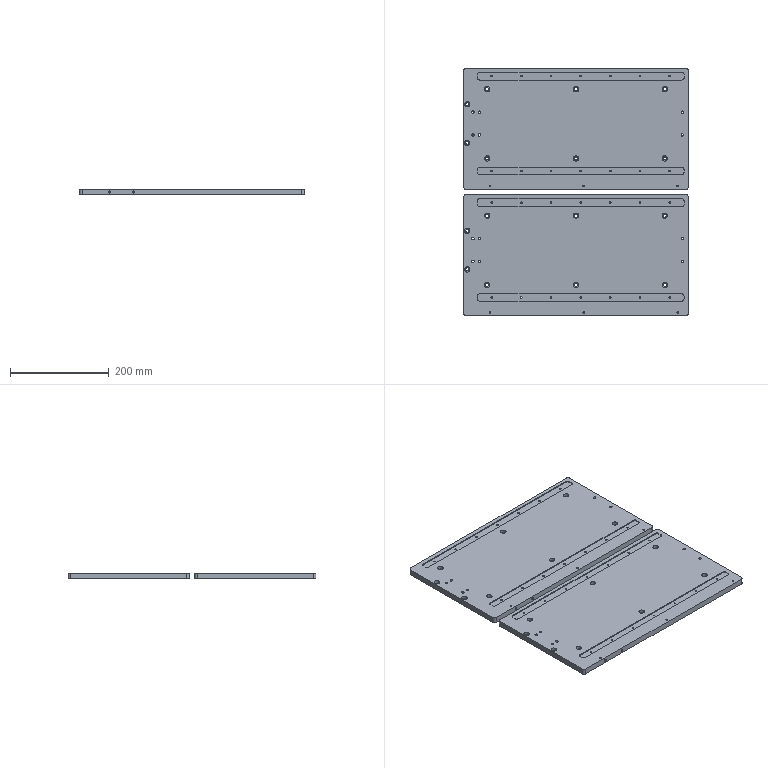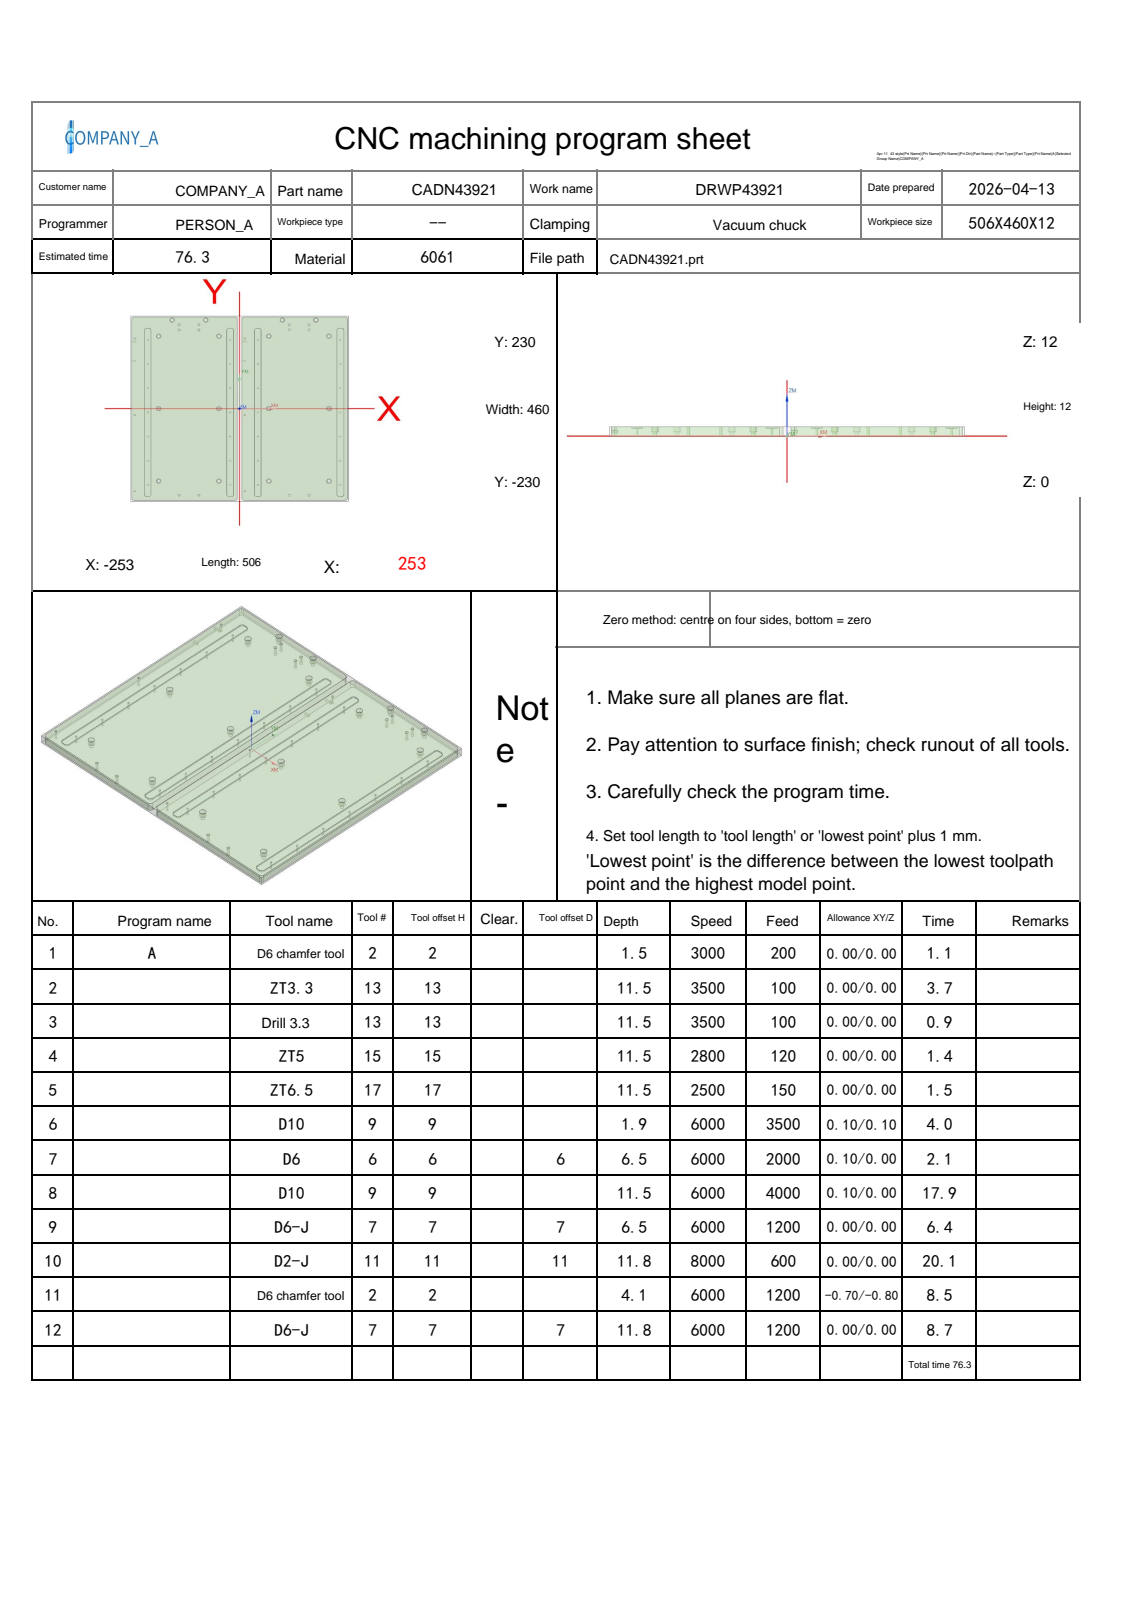NC program | NX | posted by the shop | part box 455 x 501 x 12 mm
Lines 1 to 1767 of 11580, first 1628 of 1765 lines:
%
O0001
(Machine time: 77.93 MIN)
(===Total Tool:8===)
(T2=D6 chamfer tool   D=6.   R=0.   D-  H02 Z=7.85  )
(T13=ZT3.3  D=3.3  DR_a=118 D-  H13 Z=0.5   )
(T15=ZT5    D=5.   DR_a=118 D-  H15 Z=0.5   )
(T17=ZT6.5  D=6.5  DR_a=118 D-  H17 Z=0.5   )
(T9=D10     D=10.  R=0.   D-  H09 Z=0.5   )
(T6=D6      D=6.   R=0.   D6  H06 Z=5.5   )
(T7=D6-J    D=6.   R=0.   D7  H07 Z=0.2   )
(T11=D2-J   D=2.   R=0.   D11 H11 Z=0.2   )
G80 G90 G17 G49 G40
G91 G28 Z0
M01
N1 T02 M06
(D6 chamfer tool  D=6. R=0. H=02 ce=0.00 di=0.00)
G00 G90 G54 X42.5 Y-129.5 M03 S3000
G43 H02 Z32.
M08
G98 G81 X42.5 Y-129.5 Z10.5 R13. F200.
Y-69.5
X12. Y-15.678
X42.5 Y-9.5
X68. Y0.0
X42.5 Y50.5
Y110.5
X-21.5
Y50.5
X-48. Y0.0
X-21.5 Y-9.5
Y-69.5
Y-129.5
X-48. Y-180.
X-21.5 Y-189.5
X12. Y-205.678
X42.5 Y-189.5
X68. Y-180.
X115.5 Y-215.
X161.5
X208. Y-180.
X234.5 Y-189.5
Y-129.5
Y-69.5
Y-9.5
X208. Y0.0
X234.5 Y50.5
Y110.5
Y170.5
X208. Y180.
X177.5 Y220.
X161.5 Y208.5
Y195.5
X115.5
Y208.5
X99.5 Y220.
X68. Y180.
X42.5 Y170.5
X12. Y174.322
X-21.5 Y170.5
X-48. Y180.
X-78.5 Y220.
X-94.5 Y208.5
Y195.5
X-140.5
Y208.5
X-156.5 Y220.
X-188. Y180.
X-213.5 Y170.5
X-244. Y174.322
X-213.5 Y110.5
Y50.5
X-188. Y0.0
X-213.5 Y-9.5
X-244. Y-15.678
X-213.5 Y-69.5
Y-129.5
X-244. Y-205.678
X-213.5 Y-189.5
X-188. Y-180.
X-140.5 Y-215.
X-94.5
G80
G00 Z32.
G91 G28 Z0.0
M05
M09
G91 G28 Z0.0
M01
N2 T13 M06
(ZT3.3 D=3.3 DR_a=118 H=13)
G00 G90 G54 X-213.5 Y-189.5 M03 S3500
G43 H13 Z32.
M08
G98 G83 X-213.5 Y-189.5 Z.5 R13. F100. Q1.5
Y-129.5
Y-69.5
Y-9.5
Y50.5
Y110.5
Y170.5
X-21.5 Y110.5
Y170.5
X42.5
Y110.5
Y50.5
X-21.5
Y-9.5
X42.5
Y-69.5
X-21.5
Y-129.5
Y-189.5
X42.5
Y-129.5
X234.5 Y-189.5
Y-129.5
Y-69.5
Y-9.5
Y50.5
Y110.5
Y170.5
G80
G00 Z32.
G91 G28 Z0.0
M05
M09
G91 G28 Z0.0
M01
N3 T13 M06
(Drill 3.3 D=3.3 DR_a=118 H=13)
G00 G90 G54 X-244. Y-205.678 M03 S3500
G43 H13 Z32.
M08
G98 G83 X-244. Y-205.678 Z.5 R13. F100. Q1.5
Y-15.678
Y174.322
X12.
Y-15.678
Y-205.678
G80
G00 Z32.
G91 G28 Z0.0
M05
M09
G91 G28 Z0.0
M01
N4 T15 M06
(ZT5 D=5. DR_a=118 H=15)
G00 G90 G54 X161.5 Y195.5 M03 S2800
G43 H15 Z32.
M08
G98 G83 X161.5 Y195.5 Z.5 R13. F120. Q1.5
Y208.5
X115.5
Y195.5
X-94.5
Y208.5
X-140.5
Y195.5
Y-215.
X-94.5
X115.5
X161.5
G80
G00 Z32.
G91 G28 Z0.0
M05
M09
G91 G28 Z0.0
M01
N5 T17 M06
(ZT6.5 D=6.5 DR_a=118 H=17)
G00 G90 G54 X-188. Y180. M03 S2500
G43 H17 Z32.
M08
G98 G83 X-188. Y180. Z.5 R13. F150. Q3.
X-156.5 Y220.
X-78.5
X-48. Y180.
X68.
X99.5 Y220.
X177.5
X208. Y180.
Y0.0
X68.
X-48.
X-188.
Y-180.
X-48.
X68.
X208.
G80
G00 Z32.
G91 G28 Z0.0
M05
M09
G91 G28 Z0.0
M01
N6 T09 M06
(D10  D=10. R=0. H=09 ce=0.10 di=0.10)
G00 G90 G54 X237.1 Y-37.42 M03 S6000
G43 H09 Z32.
M08
Z12.5
M03 S6000
G01 Y-9.5 Z11.525 F2800.
X237.4
M03 S6000
Y194.5 F3500.
X237.395 Y194.555
X237.355 Y194.595
X237.3 Y194.6
X231.689 Y194.599
X231.638 Y194.591
X231.603 Y194.551
X231.6 Y194.5
Y-213.5
X231.605 Y-213.555
X231.645 Y-213.595
X231.7 Y-213.6
X237.3
X237.355 Y-213.595
X237.395 Y-213.555
X237.4 Y-213.5
Y-9.5
Z12.525
G00 Z13.
X237.1 Y-37.42
Z12.025
M03 S6000
G01 Y-9.5 Z11.05 F2800.
X237.4
M03 S6000
Y194.5 F3500.
X237.395 Y194.555
X237.355 Y194.595
X237.3 Y194.6
X231.689 Y194.599
X231.638 Y194.591
X231.603 Y194.551
X231.6 Y194.5
Y-213.5
X231.605 Y-213.555
X231.645 Y-213.595
X231.7 Y-213.6
X237.3
X237.355 Y-213.595
X237.395 Y-213.555
X237.4 Y-213.5
Y-9.5
Z12.05
G00 Z12.525
X237.1 Y-37.42
Z11.55
M03 S6000
G01 Y-9.5 Z10.575 F2800.
X237.4
M03 S6000
Y194.5 F3500.
X237.395 Y194.555
X237.355 Y194.595
X237.3 Y194.6
X231.689 Y194.599
X231.638 Y194.591
X231.603 Y194.551
X231.6 Y194.5
Y-213.5
X231.605 Y-213.555
X231.645 Y-213.595
X231.7 Y-213.6
X237.3
X237.355 Y-213.595
X237.395 Y-213.555
X237.4 Y-213.5
Y-9.5
Z11.575
G00 Z12.05
X237.1 Y-37.42
Z11.075
M03 S6000
G01 Y-9.5 Z10.1 F2800.
X237.4
M03 S6000
Y194.5 F3500.
X237.395 Y194.555
X237.355 Y194.595
X237.3 Y194.6
X231.689 Y194.599
X231.638 Y194.591
X231.603 Y194.551
X231.6 Y194.5
Y-213.5
X231.605 Y-213.555
X231.645 Y-213.595
X231.7 Y-213.6
X237.3
X237.355 Y-213.595
X237.395 Y-213.555
X237.4 Y-213.5
Y-9.5
Z11.1
G00 Z32.
X44.65 Y-37.42
Z12.5
M03 S6000
G01 Y-9.5 Z11.525 F2800.
X44.95
M03 S6000
Y194.45 F3500.
X40.05
Y-213.45
X44.95
Y-9.5
Z12.525
G00 Z13.
X44.65 Y-37.42
Z12.025
M03 S6000
G01 Y-9.5 Z11.05 F2800.
X44.95
M03 S6000
Y194.45 F3500.
X40.05
Y-213.45
X44.95
Y-9.5
Z12.05
G00 Z12.525
X44.65 Y-37.42
Z11.55
M03 S6000
G01 Y-9.5 Z10.575 F2800.
X44.95
M03 S6000
Y194.45 F3500.
X40.05
Y-213.45
X44.95
Y-9.5
Z11.575
G00 Z12.05
X44.65 Y-37.42
Z11.075
M03 S6000
G01 Y-9.5 Z10.1 F2800.
X44.95
M03 S6000
Y194.45 F3500.
X40.05
Y-213.45
X44.95
Y-9.5
Z11.1
G00 Z32.
X-18.9 Y-37.42
Z12.5
M03 S6000
G01 Y-9.5 Z11.525 F2800.
X-18.6
M03 S6000
Y194.5 F3500.
X-18.605 Y194.555
X-18.645 Y194.595
X-18.7 Y194.6
X-24.3
X-24.355 Y194.595
X-24.395 Y194.555
X-24.4 Y194.5
Y-213.5
X-24.403 Y-213.539
X-24.375 Y-213.567
X-24.357 Y-213.594
X-24.328 Y-213.606
X-24.296 Y-213.6
X-18.7
X-18.645 Y-213.595
X-18.605 Y-213.555
X-18.6 Y-213.5
Y-9.5
Z12.525
G00 Z13.
X-18.9 Y-37.42
Z12.025
M03 S6000
G01 Y-9.5 Z11.05 F2800.
X-18.6
M03 S6000
Y194.5 F3500.
X-18.605 Y194.555
X-18.645 Y194.595
X-18.7 Y194.6
X-24.3
X-24.355 Y194.595
X-24.395 Y194.555
X-24.4 Y194.5
Y-213.5
X-24.395 Y-213.555
X-24.355 Y-213.595
X-24.3 Y-213.6
X-18.7
X-18.645 Y-213.595
X-18.605 Y-213.555
X-18.6 Y-213.5
Y-9.5
Z12.05
G00 Z12.525
X-18.9 Y-37.42
Z11.55
M03 S6000
G01 Y-9.5 Z10.575 F2800.
X-18.6
M03 S6000
Y194.5 F3500.
X-18.605 Y194.555
X-18.645 Y194.595
X-18.7 Y194.6
X-24.3
X-24.355 Y194.595
X-24.395 Y194.555
X-24.4 Y194.5
Y-213.5
X-24.395 Y-213.555
X-24.355 Y-213.595
X-24.3 Y-213.6
X-18.7
X-18.645 Y-213.595
X-18.605 Y-213.555
X-18.6 Y-213.5
Y-9.5
Z11.575
G00 Z12.05
X-18.9 Y-37.42
Z11.075
M03 S6000
G01 Y-9.5 Z10.1 F2800.
X-18.6
M03 S6000
Y194.5 F3500.
X-18.605 Y194.555
X-18.645 Y194.595
X-18.7 Y194.6
X-24.3
X-24.355 Y194.595
X-24.395 Y194.555
X-24.4 Y194.5
Y-213.5
X-24.395 Y-213.555
X-24.355 Y-213.595
X-24.3 Y-213.6
X-18.7
X-18.645 Y-213.595
X-18.605 Y-213.555
X-18.6 Y-213.5
Y-9.5
Z11.1
G00 Z32.
X-215.65 Y18.42
Z12.5
M03 S6000
G01 Y-9.5 Z11.525 F2800.
X-215.95
M03 S6000
Y-213.45 F3500.
X-211.05
Y194.45
X-215.95
Y-9.5
Z12.525
G00 Z13.
X-215.65 Y18.42
Z12.025
M03 S6000
G01 Y-9.5 Z11.05 F2800.
X-215.95
M03 S6000
Y-213.45 F3500.
X-211.05
Y194.45
X-215.95
Y-9.5
Z12.05
G00 Z12.525
X-215.65 Y18.42
Z11.55
M03 S6000
G01 Y-9.5 Z10.575 F2800.
X-215.95
M03 S6000
Y-213.45 F3500.
X-211.05
Y194.45
X-215.95
Y-9.5
Z11.575
G00 Z12.05
X-215.65 Y18.42
Z11.075
M03 S6000
G01 Y-9.5 Z10.1 F2800.
X-215.95
M03 S6000
Y-213.45 F3500.
X-211.05
Y194.45
X-215.95
Y-9.5
Z11.1
G00 Z32.
G91 G28 Z0.0
M05
M09
G91 G28 Z0.0
M01
N7 T06 M06
(D6  D=6. R=0. H=06 ce=0.10 di=0.00)
G00 G90 G54 X-156.5 Y220. M03 S6000
G43 H06 Z32.
M08
Z12.3
G41 D06
G01 X-156.6 Y219.992 F2000.
G03 X-157.698 Y218.798 I.1 J-1.194
X-156.5 Y217.6 I1.198 J0.0
X-156.5 Y217.6 Z11.8 I0.0 J2.4
X-156.5 Y217.6 Z11.3 I0.0 J2.4
X-156.5 Y217.6 Z10.8 I0.0 J2.4
X-156.5 Y217.6 Z10.3 I0.0 J2.4
X-156.5 Y217.6 Z9.8 I0.0 J2.4
X-156.5 Y217.6 Z9.3 I0.0 J2.4
X-156.5 Y217.6 Z8.8 I0.0 J2.4
X-156.5 Y217.6 Z8.3 I0.0 J2.4
X-156.5 Y217.6 Z7.8 I0.0 J2.4
X-156.5 Y217.6 Z7.3 I0.0 J2.4
X-156.5 Y217.6 Z6.8 I0.0 J2.4
X-156.5 Y217.6 Z6.3 I0.0 J2.4
X-156.5 Y217.6 Z5.8 I0.0 J2.4
X-157.911 Y221.942 Z5.5 I0.0 J2.4
X-158.9 Y220. I1.411 J-1.942
X-156.5 Y217.6 I2.4 J0.0
X-154.1 Y220. I0.0 J2.4
X-156.5 Y222.4 I-2.4 J0.0
X-157.911 Y221.942 I0.0 J-2.4
X-158.404 Y220.973 I.704 J-.969
X-157.207 Y219.775 I1.198 J0.0
X-156.586 Y219.948 I0.0 J1.198
G01 G40 X-156.5 Y220.
G00 Z32.
X-188. Y180.
Z12.3
G41 D06
G01 X-188.1 Y179.992
G03 X-189.198 Y178.798 I.1 J-1.194
X-188. Y177.6 I1.198 J0.0
X-188. Y177.6 Z11.8 I0.0 J2.4
X-188. Y177.6 Z11.3 I0.0 J2.4
X-188. Y177.6 Z10.8 I0.0 J2.4
X-188. Y177.6 Z10.3 I0.0 J2.4
X-188. Y177.6 Z9.8 I0.0 J2.4
X-188. Y177.6 Z9.3 I0.0 J2.4
X-188. Y177.6 Z8.8 I0.0 J2.4
X-188. Y177.6 Z8.3 I0.0 J2.4
X-188. Y177.6 Z7.8 I0.0 J2.4
X-188. Y177.6 Z7.3 I0.0 J2.4
X-188. Y177.6 Z6.8 I0.0 J2.4
X-188. Y177.6 Z6.3 I0.0 J2.4
X-188. Y177.6 Z5.8 I0.0 J2.4
X-189.411 Y181.942 Z5.5 I0.0 J2.4
X-190.4 Y180. I1.411 J-1.942
X-188. Y177.6 I2.4 J0.0
X-185.6 Y180. I0.0 J2.4
X-188. Y182.4 I-2.4 J0.0
X-189.411 Y181.942 I0.0 J-2.4
X-189.904 Y180.973 I.704 J-.969
X-188.707 Y179.775 I1.198 J0.0
X-188.086 Y179.948 I0.0 J1.198
G01 G40 X-188. Y180.
G00 Z32.
X-78.5 Y220.
Z12.3
G41 D06
G01 X-78.6 Y219.992
G03 X-79.698 Y218.798 I.1 J-1.194
X-78.5 Y217.6 I1.198 J0.0
X-78.5 Y217.6 Z11.8 I0.0 J2.4
X-78.5 Y217.6 Z11.3 I0.0 J2.4
X-78.5 Y217.6 Z10.8 I0.0 J2.4
X-78.5 Y217.6 Z10.3 I0.0 J2.4
X-78.5 Y217.6 Z9.8 I0.0 J2.4
X-78.5 Y217.6 Z9.3 I0.0 J2.4
X-78.5 Y217.6 Z8.8 I0.0 J2.4
X-78.5 Y217.6 Z8.3 I0.0 J2.4
X-78.5 Y217.6 Z7.8 I0.0 J2.4
X-78.5 Y217.6 Z7.3 I0.0 J2.4
X-78.5 Y217.6 Z6.8 I0.0 J2.4
X-78.5 Y217.6 Z6.3 I0.0 J2.4
X-78.5 Y217.6 Z5.8 I0.0 J2.4
X-79.911 Y221.942 Z5.5 I0.0 J2.4
X-80.9 Y220. I1.411 J-1.942
X-78.5 Y217.6 I2.4 J0.0
X-76.1 Y220. I0.0 J2.4
X-78.5 Y222.4 I-2.4 J0.0
X-79.911 Y221.942 I0.0 J-2.4
X-80.404 Y220.973 I.704 J-.969
X-79.207 Y219.775 I1.198 J0.0
X-78.586 Y219.948 I0.0 J1.198
G01 G40 X-78.5 Y220.
G00 Z32.
X-48. Y180.
Z12.3
G41 D06
G01 X-48.1 Y179.992
G03 X-49.198 Y178.798 I.1 J-1.194
X-48. Y177.6 I1.198 J0.0
X-48. Y177.6 Z11.8 I0.0 J2.4
X-48. Y177.6 Z11.3 I0.0 J2.4
X-48. Y177.6 Z10.8 I0.0 J2.4
X-48. Y177.6 Z10.3 I0.0 J2.4
X-48. Y177.6 Z9.8 I0.0 J2.4
X-48. Y177.6 Z9.3 I0.0 J2.4
X-48. Y177.6 Z8.8 I0.0 J2.4
X-48. Y177.6 Z8.3 I0.0 J2.4
X-48. Y177.6 Z7.8 I0.0 J2.4
X-48. Y177.6 Z7.3 I0.0 J2.4
X-48. Y177.6 Z6.8 I0.0 J2.4
X-48. Y177.6 Z6.3 I0.0 J2.4
X-48. Y177.6 Z5.8 I0.0 J2.4
X-49.411 Y181.942 Z5.5 I0.0 J2.4
X-50.4 Y180. I1.411 J-1.942
X-48. Y177.6 I2.4 J0.0
X-45.6 Y180. I0.0 J2.4
X-48. Y182.4 I-2.4 J0.0
X-49.411 Y181.942 I0.0 J-2.4
X-49.904 Y180.973 I.704 J-.969
X-48.707 Y179.775 I1.198 J0.0
X-48.086 Y179.948 I0.0 J1.198
G01 G40 X-48. Y180.
G00 Z32.
X68.
Z12.3
G41 D06
G01 X67.9 Y179.992
G03 X66.802 Y178.798 I.1 J-1.194
X68. Y177.6 I1.198 J0.0
X68. Y177.6 Z11.8 I0.0 J2.4
X68. Y177.6 Z11.3 I0.0 J2.4
X68. Y177.6 Z10.8 I0.0 J2.4
X68. Y177.6 Z10.3 I0.0 J2.4
X68. Y177.6 Z9.8 I0.0 J2.4
X68. Y177.6 Z9.3 I0.0 J2.4
X68. Y177.6 Z8.8 I0.0 J2.4
X68. Y177.6 Z8.3 I0.0 J2.4
X68. Y177.6 Z7.8 I0.0 J2.4
X68. Y177.6 Z7.3 I0.0 J2.4
X68. Y177.6 Z6.8 I0.0 J2.4
X68. Y177.6 Z6.3 I0.0 J2.4
X68. Y177.6 Z5.8 I0.0 J2.4
X66.589 Y181.942 Z5.5 I0.0 J2.4
X65.6 Y180. I1.411 J-1.942
X68. Y177.6 I2.4 J0.0
X70.4 Y180. I0.0 J2.4
X68. Y182.4 I-2.4 J0.0
X66.589 Y181.942 I0.0 J-2.4
X66.096 Y180.973 I.704 J-.969
X67.293 Y179.775 I1.198 J0.0
X67.914 Y179.948 I0.0 J1.198
G01 G40 X68. Y180.
G00 Z32.
X99.5 Y220.
Z12.3
G41 D06
G01 X99.4 Y219.992
G03 X98.302 Y218.798 I.1 J-1.194
X99.5 Y217.6 I1.198 J0.0
X99.5 Y217.6 Z11.8 I0.0 J2.4
X99.5 Y217.6 Z11.3 I0.0 J2.4
X99.5 Y217.6 Z10.8 I0.0 J2.4
X99.5 Y217.6 Z10.3 I0.0 J2.4
X99.5 Y217.6 Z9.8 I0.0 J2.4
X99.5 Y217.6 Z9.3 I0.0 J2.4
X99.5 Y217.6 Z8.8 I0.0 J2.4
X99.5 Y217.6 Z8.3 I0.0 J2.4
X99.5 Y217.6 Z7.8 I0.0 J2.4
X99.5 Y217.6 Z7.3 I0.0 J2.4
X99.5 Y217.6 Z6.8 I0.0 J2.4
X99.5 Y217.6 Z6.3 I0.0 J2.4
X99.5 Y217.6 Z5.8 I0.0 J2.4
X98.089 Y221.942 Z5.5 I0.0 J2.4
X97.1 Y220. I1.411 J-1.942
X99.5 Y217.6 I2.4 J0.0
X101.9 Y220. I0.0 J2.4
X99.5 Y222.4 I-2.4 J0.0
X98.089 Y221.942 I0.0 J-2.4
X97.596 Y220.973 I.704 J-.969
X98.793 Y219.775 I1.198 J0.0
X99.414 Y219.948 I0.0 J1.198
G01 G40 X99.5 Y220.
G00 Z32.
X177.5
Z12.3
G41 D06
G01 X177.4 Y219.992
G03 X176.302 Y218.798 I.1 J-1.194
X177.5 Y217.6 I1.198 J0.0
X177.5 Y217.6 Z11.8 I0.0 J2.4
X177.5 Y217.6 Z11.3 I0.0 J2.4
X177.5 Y217.6 Z10.8 I0.0 J2.4
X177.5 Y217.6 Z10.3 I0.0 J2.4
X177.5 Y217.6 Z9.8 I0.0 J2.4
X177.5 Y217.6 Z9.3 I0.0 J2.4
X177.5 Y217.6 Z8.8 I0.0 J2.4
X177.5 Y217.6 Z8.3 I0.0 J2.4
X177.5 Y217.6 Z7.8 I0.0 J2.4
X177.5 Y217.6 Z7.3 I0.0 J2.4
X177.5 Y217.6 Z6.8 I0.0 J2.4
X177.5 Y217.6 Z6.3 I0.0 J2.4
X177.5 Y217.6 Z5.8 I0.0 J2.4
X176.089 Y221.942 Z5.5 I0.0 J2.4
X175.1 Y220. I1.411 J-1.942
X177.5 Y217.6 I2.4 J0.0
X179.9 Y220. I0.0 J2.4
X177.5 Y222.4 I-2.4 J0.0
X176.089 Y221.942 I0.0 J-2.4
X175.596 Y220.973 I.704 J-.969
X176.793 Y219.775 I1.198 J0.0
X177.414 Y219.948 I0.0 J1.198
G01 G40 X177.5 Y220.
G00 Z32.
X208. Y180.
Z12.3
G41 D06
G01 X207.9 Y179.992
G03 X206.802 Y178.798 I.1 J-1.194
X208. Y177.6 I1.198 J0.0
X208. Y177.6 Z11.8 I0.0 J2.4
X208. Y177.6 Z11.3 I0.0 J2.4
X208. Y177.6 Z10.8 I0.0 J2.4
X208. Y177.6 Z10.3 I0.0 J2.4
X208. Y177.6 Z9.8 I0.0 J2.4
X208. Y177.6 Z9.3 I0.0 J2.4
X208. Y177.6 Z8.8 I0.0 J2.4
X208. Y177.6 Z8.3 I0.0 J2.4
X208. Y177.6 Z7.8 I0.0 J2.4
X208. Y177.6 Z7.3 I0.0 J2.4
X208. Y177.6 Z6.8 I0.0 J2.4
X208. Y177.6 Z6.3 I0.0 J2.4
X208. Y177.6 Z5.8 I0.0 J2.4
X206.589 Y181.942 Z5.5 I0.0 J2.4
X205.6 Y180. I1.411 J-1.942
X208. Y177.6 I2.4 J0.0
X210.4 Y180. I0.0 J2.4
X208. Y182.4 I-2.4 J0.0
X206.589 Y181.942 I0.0 J-2.4
X206.096 Y180.973 I.704 J-.969
X207.293 Y179.775 I1.198 J0.0
X207.914 Y179.948 I0.0 J1.198
G01 G40 X208. Y180.
G00 Z32.
Y0.0
Z12.3
G41 D06
G01 X207.9 Y-.008
G03 X206.802 Y-1.202 I.1 J-1.194
X208. Y-2.4 I1.198 J0.0
X208. Y-2.4 Z11.8 I0.0 J2.4
X208. Y-2.4 Z11.3 I0.0 J2.4
X208. Y-2.4 Z10.8 I0.0 J2.4
X208. Y-2.4 Z10.3 I0.0 J2.4
X208. Y-2.4 Z9.8 I0.0 J2.4
X208. Y-2.4 Z9.3 I0.0 J2.4
X208. Y-2.4 Z8.8 I0.0 J2.4
X208. Y-2.4 Z8.3 I0.0 J2.4
X208. Y-2.4 Z7.8 I0.0 J2.4
X208. Y-2.4 Z7.3 I0.0 J2.4
X208. Y-2.4 Z6.8 I0.0 J2.4
X208. Y-2.4 Z6.3 I0.0 J2.4
X208. Y-2.4 Z5.8 I0.0 J2.4
X206.589 Y1.942 Z5.5 I0.0 J2.4
X205.6 Y0.0 I1.411 J-1.942
X208. Y-2.4 I2.4 J0.0
X210.4 Y0.0 I0.0 J2.4
X208. Y2.4 I-2.4 J0.0
X206.589 Y1.942 I0.0 J-2.4
X206.096 Y.973 I.704 J-.969
X207.293 Y-.225 I1.198 J0.0
X207.914 Y-.052 I0.0 J1.198
G01 G40 X208. Y0.0
G00 Z32.
X68.
Z12.3
G41 D06
G01 X67.9 Y-.008
G03 X66.802 Y-1.202 I.1 J-1.194
X68. Y-2.4 I1.198 J0.0
X68. Y-2.4 Z11.8 I0.0 J2.4
X68. Y-2.4 Z11.3 I0.0 J2.4
X68. Y-2.4 Z10.8 I0.0 J2.4
X68. Y-2.4 Z10.3 I0.0 J2.4
X68. Y-2.4 Z9.8 I0.0 J2.4
X68. Y-2.4 Z9.3 I0.0 J2.4
X68. Y-2.4 Z8.8 I0.0 J2.4
X68. Y-2.4 Z8.3 I0.0 J2.4
X68. Y-2.4 Z7.8 I0.0 J2.4
X68. Y-2.4 Z7.3 I0.0 J2.4
X68. Y-2.4 Z6.8 I0.0 J2.4
X68. Y-2.4 Z6.3 I0.0 J2.4
X68. Y-2.4 Z5.8 I0.0 J2.4
X66.589 Y1.942 Z5.5 I0.0 J2.4
X65.6 Y0.0 I1.411 J-1.942
X68. Y-2.4 I2.4 J0.0
X70.4 Y0.0 I0.0 J2.4
X68. Y2.4 I-2.4 J0.0
X66.589 Y1.942 I0.0 J-2.4
X66.096 Y.973 I.704 J-.969
X67.293 Y-.225 I1.198 J0.0
X67.914 Y-.052 I0.0 J1.198
G01 G40 X68. Y0.0
G00 Z32.
X-48.
Z12.3
G41 D06
G01 X-48.1 Y-.008
G03 X-49.198 Y-1.202 I.1 J-1.194
X-48. Y-2.4 I1.198 J0.0
X-48. Y-2.4 Z11.8 I0.0 J2.4
X-48. Y-2.4 Z11.3 I0.0 J2.4
X-48. Y-2.4 Z10.8 I0.0 J2.4
X-48. Y-2.4 Z10.3 I0.0 J2.4
X-48. Y-2.4 Z9.8 I0.0 J2.4
X-48. Y-2.4 Z9.3 I0.0 J2.4
X-48. Y-2.4 Z8.8 I0.0 J2.4
X-48. Y-2.4 Z8.3 I0.0 J2.4
X-48. Y-2.4 Z7.8 I0.0 J2.4
X-48. Y-2.4 Z7.3 I0.0 J2.4
X-48. Y-2.4 Z6.8 I0.0 J2.4
X-48. Y-2.4 Z6.3 I0.0 J2.4
X-48. Y-2.4 Z5.8 I0.0 J2.4
X-49.411 Y1.942 Z5.5 I0.0 J2.4
X-50.4 Y0.0 I1.411 J-1.942
X-48. Y-2.4 I2.4 J0.0
X-45.6 Y0.0 I0.0 J2.4
X-48. Y2.4 I-2.4 J0.0
X-49.411 Y1.942 I0.0 J-2.4
X-49.904 Y.973 I.704 J-.969
X-48.707 Y-.225 I1.198 J0.0
X-48.086 Y-.052 I0.0 J1.198
G01 G40 X-48. Y0.0
G00 Z32.
X-188.
Z12.3
G41 D06
G01 X-188.1 Y-.008
G03 X-189.198 Y-1.202 I.1 J-1.194
X-188. Y-2.4 I1.198 J0.0
X-188. Y-2.4 Z11.8 I0.0 J2.4
X-188. Y-2.4 Z11.3 I0.0 J2.4
X-188. Y-2.4 Z10.8 I0.0 J2.4
X-188. Y-2.4 Z10.3 I0.0 J2.4
X-188. Y-2.4 Z9.8 I0.0 J2.4
X-188. Y-2.4 Z9.3 I0.0 J2.4
X-188. Y-2.4 Z8.8 I0.0 J2.4
X-188. Y-2.4 Z8.3 I0.0 J2.4
X-188. Y-2.4 Z7.8 I0.0 J2.4
X-188. Y-2.4 Z7.3 I0.0 J2.4
X-188. Y-2.4 Z6.8 I0.0 J2.4
X-188. Y-2.4 Z6.3 I0.0 J2.4
X-188. Y-2.4 Z5.8 I0.0 J2.4
X-189.411 Y1.942 Z5.5 I0.0 J2.4
X-190.4 Y0.0 I1.411 J-1.942
X-188. Y-2.4 I2.4 J0.0
X-185.6 Y0.0 I0.0 J2.4
X-188. Y2.4 I-2.4 J0.0
X-189.411 Y1.942 I0.0 J-2.4
X-189.904 Y.973 I.704 J-.969
X-188.707 Y-.225 I1.198 J0.0
X-188.086 Y-.052 I0.0 J1.198
G01 G40 X-188. Y0.0
G00 Z32.
Y-180.
Z12.3
G41 D06
G01 X-188.1 Y-180.008
G03 X-189.198 Y-181.202 I.1 J-1.194
X-188. Y-182.4 I1.198 J0.0
X-188. Y-182.4 Z11.8 I0.0 J2.4
X-188. Y-182.4 Z11.3 I0.0 J2.4
X-188. Y-182.4 Z10.8 I0.0 J2.4
X-188. Y-182.4 Z10.3 I0.0 J2.4
X-188. Y-182.4 Z9.8 I0.0 J2.4
X-188. Y-182.4 Z9.3 I0.0 J2.4
X-188. Y-182.4 Z8.8 I0.0 J2.4
X-188. Y-182.4 Z8.3 I0.0 J2.4
X-188. Y-182.4 Z7.8 I0.0 J2.4
X-188. Y-182.4 Z7.3 I0.0 J2.4
X-188. Y-182.4 Z6.8 I0.0 J2.4
X-188. Y-182.4 Z6.3 I0.0 J2.4
X-188. Y-182.4 Z5.8 I0.0 J2.4
X-189.411 Y-178.058 Z5.5 I0.0 J2.4
X-190.4 Y-180. I1.411 J-1.942
X-188. Y-182.4 I2.4 J0.0
X-185.6 Y-180. I0.0 J2.4
X-188. Y-177.6 I-2.4 J0.0
X-189.411 Y-178.058 I0.0 J-2.4
X-189.904 Y-179.027 I.704 J-.969
X-188.707 Y-180.225 I1.198 J0.0
X-188.086 Y-180.052 I0.0 J1.198
G01 G40 X-188. Y-180.
G00 Z32.
X-48.
Z12.3
G41 D06
G01 X-48.1 Y-180.008
G03 X-49.198 Y-181.202 I.1 J-1.194
X-48. Y-182.4 I1.198 J0.0
X-48. Y-182.4 Z11.8 I0.0 J2.4
X-48. Y-182.4 Z11.3 I0.0 J2.4
X-48. Y-182.4 Z10.8 I0.0 J2.4
X-48. Y-182.4 Z10.3 I0.0 J2.4
X-48. Y-182.4 Z9.8 I0.0 J2.4
X-48. Y-182.4 Z9.3 I0.0 J2.4
X-48. Y-182.4 Z8.8 I0.0 J2.4
X-48. Y-182.4 Z8.3 I0.0 J2.4
X-48. Y-182.4 Z7.8 I0.0 J2.4
X-48. Y-182.4 Z7.3 I0.0 J2.4
X-48. Y-182.4 Z6.8 I0.0 J2.4
X-48. Y-182.4 Z6.3 I0.0 J2.4
X-48. Y-182.4 Z5.8 I0.0 J2.4
X-49.411 Y-178.058 Z5.5 I0.0 J2.4
X-50.4 Y-180. I1.411 J-1.942
X-48. Y-182.4 I2.4 J0.0
X-45.6 Y-180. I0.0 J2.4
X-48. Y-177.6 I-2.4 J0.0
X-49.411 Y-178.058 I0.0 J-2.4
X-49.904 Y-179.027 I.704 J-.969
X-48.707 Y-180.225 I1.198 J0.0
X-48.086 Y-180.052 I0.0 J1.198
G01 G40 X-48. Y-180.
G00 Z32.
X68.
Z12.3
G41 D06
G01 X67.9 Y-180.008
G03 X66.802 Y-181.202 I.1 J-1.194
X68. Y-182.4 I1.198 J0.0
X68. Y-182.4 Z11.8 I0.0 J2.4
X68. Y-182.4 Z11.3 I0.0 J2.4
X68. Y-182.4 Z10.8 I0.0 J2.4
X68. Y-182.4 Z10.3 I0.0 J2.4
X68. Y-182.4 Z9.8 I0.0 J2.4
X68. Y-182.4 Z9.3 I0.0 J2.4
X68. Y-182.4 Z8.8 I0.0 J2.4
X68. Y-182.4 Z8.3 I0.0 J2.4
X68. Y-182.4 Z7.8 I0.0 J2.4
X68. Y-182.4 Z7.3 I0.0 J2.4
X68. Y-182.4 Z6.8 I0.0 J2.4
X68. Y-182.4 Z6.3 I0.0 J2.4
X68. Y-182.4 Z5.8 I0.0 J2.4
X66.589 Y-178.058 Z5.5 I0.0 J2.4
X65.6 Y-180. I1.411 J-1.942
X68. Y-182.4 I2.4 J0.0
X70.4 Y-180. I0.0 J2.4
X68. Y-177.6 I-2.4 J0.0
X66.589 Y-178.058 I0.0 J-2.4
X66.096 Y-179.027 I.704 J-.969
X67.293 Y-180.225 I1.198 J0.0
X67.914 Y-180.052 I0.0 J1.198
G01 G40 X68. Y-180.
G00 Z32.
X208.
Z12.3
G41 D06
G01 X207.9 Y-180.008
G03 X206.802 Y-181.202 I.1 J-1.194
X208. Y-182.4 I1.198 J0.0
X208. Y-182.4 Z11.8 I0.0 J2.4
X208. Y-182.4 Z11.3 I0.0 J2.4
X208. Y-182.4 Z10.8 I0.0 J2.4
X208. Y-182.4 Z10.3 I0.0 J2.4
X208. Y-182.4 Z9.8 I0.0 J2.4
X208. Y-182.4 Z9.3 I0.0 J2.4
X208. Y-182.4 Z8.8 I0.0 J2.4
X208. Y-182.4 Z8.3 I0.0 J2.4
X208. Y-182.4 Z7.8 I0.0 J2.4
X208. Y-182.4 Z7.3 I0.0 J2.4
X208. Y-182.4 Z6.8 I0.0 J2.4
X208. Y-182.4 Z6.3 I0.0 J2.4
X208. Y-182.4 Z5.8 I0.0 J2.4
X206.589 Y-178.058 Z5.5 I0.0 J2.4
X205.6 Y-180. I1.411 J-1.942
X208. Y-182.4 I2.4 J0.0
X210.4 Y-180. I0.0 J2.4
X208. Y-177.6 I-2.4 J0.0
X206.589 Y-178.058 I0.0 J-2.4
X206.096 Y-179.027 I.704 J-.969
X207.293 Y-180.225 I1.198 J0.0
X207.914 Y-180.052 I0.0 J1.198
G01 G40 X208. Y-180.
G00 Z32.
G91 G28 Z0.0
M05
M09
G91 G28 Z0.0
M01
N8 T09 M06
(D10  D=10. R=0. H=09 ce=0.10 di=0.00)
G00 G90 G54 X255.6 Y0.0 M03 S6000
G43 H09 Z32.
M08
Z12.5
G01 Y-222.5 Z12.422 F4000.
G02 X245.5 Y-232.6 Z12.416 I-10.1 J0.0
G01 X10.5 Z12.334
G02 X.4 Y-222.5 Z12.328 I0.0 J10.1
G01 Y222.5 Z12.172
G02 X10.5 Y232.6 Z12.166 I10.1 J0.0
G01 X245.5 Z12.084
G02 X255.6 Y222.5 Z12.078 I0.0 J-10.1
G01 Y-222.5 Z11.922
G02 X245.5 Y-232.6 Z11.916 I-10.1 J0.0
G01 X10.5 Z11.834
G02 X.4 Y-222.5 Z11.828 I0.0 J10.1
G01 Y222.5 Z11.672
G02 X10.5 Y232.6 Z11.666 I10.1 J0.0
G01 X245.5 Z11.584
G02 X255.6 Y222.5 Z11.578 I0.0 J-10.1
G01 Y-222.5 Z11.422
G02 X245.5 Y-232.6 Z11.416 I-10.1 J0.0
G01 X10.5 Z11.334
G02 X.4 Y-222.5 Z11.328 I0.0 J10.1
G01 Y222.5 Z11.172
G02 X10.5 Y232.6 Z11.166 I10.1 J0.0
G01 X245.5 Z11.084
G02 X255.6 Y222.5 Z11.078 I0.0 J-10.1
G01 Y-222.5 Z10.922
G02 X245.5 Y-232.6 Z10.916 I-10.1 J0.0
G01 X10.5 Z10.834
G02 X.4 Y-222.5 Z10.828 I0.0 J10.1
G01 Y222.5 Z10.672
G02 X10.5 Y232.6 Z10.666 I10.1 J0.0
G01 X245.5 Z10.584
G02 X255.6 Y222.5 Z10.578 I0.0 J-10.1
G01 Y-222.5 Z10.422
G02 X245.5 Y-232.6 Z10.416 I-10.1 J0.0
G01 X10.5 Z10.334
G02 X.4 Y-222.5 Z10.328 I0.0 J10.1
G01 Y222.5 Z10.172
G02 X10.5 Y232.6 Z10.166 I10.1 J0.0
G01 X245.5 Z10.084
G02 X255.6 Y222.5 Z10.078 I0.0 J-10.1
G01 Y-222.5 Z9.922
G02 X245.5 Y-232.6 Z9.916 I-10.1 J0.0
G01 X10.5 Z9.834
G02 X.4 Y-222.5 Z9.828 I0.0 J10.1
G01 Y222.5 Z9.672
G02 X10.5 Y232.6 Z9.666 I10.1 J0.0
G01 X245.5 Z9.584
G02 X255.6 Y222.5 Z9.578 I0.0 J-10.1
G01 Y-222.5 Z9.422
G02 X245.5 Y-232.6 Z9.416 I-10.1 J0.0
G01 X10.5 Z9.334
G02 X.4 Y-222.5 Z9.328 I0.0 J10.1
G01 Y222.5 Z9.172
G02 X10.5 Y232.6 Z9.166 I10.1 J0.0
G01 X245.5 Z9.084
G02 X255.6 Y222.5 Z9.078 I0.0 J-10.1
G01 Y-222.5 Z8.922
G02 X245.5 Y-232.6 Z8.916 I-10.1 J0.0
G01 X10.5 Z8.834
G02 X.4 Y-222.5 Z8.828 I0.0 J10.1
G01 Y222.5 Z8.672
G02 X10.5 Y232.6 Z8.666 I10.1 J0.0
G01 X245.5 Z8.584
G02 X255.6 Y222.5 Z8.578 I0.0 J-10.1
G01 Y-222.5 Z8.422
G02 X245.5 Y-232.6 Z8.416 I-10.1 J0.0
G01 X10.5 Z8.334
G02 X.4 Y-222.5 Z8.328 I0.0 J10.1
G01 Y222.5 Z8.172
G02 X10.5 Y232.6 Z8.166 I10.1 J0.0
G01 X245.5 Z8.084
G02 X255.6 Y222.5 Z8.078 I0.0 J-10.1
G01 Y-222.5 Z7.922
G02 X245.5 Y-232.6 Z7.916 I-10.1 J0.0
G01 X10.5 Z7.834
G02 X.4 Y-222.5 Z7.828 I0.0 J10.1
G01 Y222.5 Z7.672
G02 X10.5 Y232.6 Z7.666 I10.1 J0.0
G01 X245.5 Z7.584
G02 X255.6 Y222.5 Z7.578 I0.0 J-10.1
G01 Y-222.5 Z7.422
G02 X245.5 Y-232.6 Z7.416 I-10.1 J0.0
G01 X10.5 Z7.334
G02 X.4 Y-222.5 Z7.328 I0.0 J10.1
G01 Y222.5 Z7.172
G02 X10.5 Y232.6 Z7.166 I10.1 J0.0
G01 X245.5 Z7.084
G02 X255.6 Y222.5 Z7.078 I0.0 J-10.1
G01 Y-222.5 Z6.922
G02 X245.5 Y-232.6 Z6.916 I-10.1 J0.0
G01 X10.5 Z6.834
G02 X.4 Y-222.5 Z6.828 I0.0 J10.1
G01 Y222.5 Z6.672
G02 X10.5 Y232.6 Z6.666 I10.1 J0.0
G01 X245.5 Z6.584
G02 X255.6 Y222.5 Z6.578 I0.0 J-10.1
G01 Y-222.5 Z6.422
G02 X245.5 Y-232.6 Z6.416 I-10.1 J0.0
G01 X10.5 Z6.334
G02 X.4 Y-222.5 Z6.328 I0.0 J10.1
G01 Y222.5 Z6.172
G02 X10.5 Y232.6 Z6.166 I10.1 J0.0
G01 X245.5 Z6.084
G02 X255.6 Y222.5 Z6.078 I0.0 J-10.1
G01 Y-222.5 Z5.922
G02 X245.5 Y-232.6 Z5.916 I-10.1 J0.0
G01 X10.5 Z5.834
G02 X.4 Y-222.5 Z5.828 I0.0 J10.1
G01 Y222.5 Z5.672
G02 X10.5 Y232.6 Z5.666 I10.1 J0.0
G01 X245.5 Z5.584
G02 X255.6 Y222.5 Z5.578 I0.0 J-10.1
G01 Y-222.5 Z5.422
G02 X245.5 Y-232.6 Z5.416 I-10.1 J0.0
G01 X10.5 Z5.334
G02 X.4 Y-222.5 Z5.328 I0.0 J10.1
G01 Y222.5 Z5.172
G02 X10.5 Y232.6 Z5.166 I10.1 J0.0
G01 X245.5 Z5.084
G02 X255.6 Y222.5 Z5.078 I0.0 J-10.1
G01 Y-222.5 Z4.922
G02 X245.5 Y-232.6 Z4.916 I-10.1 J0.0
G01 X10.5 Z4.834
G02 X.4 Y-222.5 Z4.828 I0.0 J10.1
G01 Y222.5 Z4.672
G02 X10.5 Y232.6 Z4.666 I10.1 J0.0
G01 X245.5 Z4.584
G02 X255.6 Y222.5 Z4.578 I0.0 J-10.1
G01 Y-222.5 Z4.422
G02 X245.5 Y-232.6 Z4.416 I-10.1 J0.0
G01 X10.5 Z4.334
G02 X.4 Y-222.5 Z4.328 I0.0 J10.1
G01 Y222.5 Z4.172
G02 X10.5 Y232.6 Z4.166 I10.1 J0.0
G01 X245.5 Z4.084
G02 X255.6 Y222.5 Z4.078 I0.0 J-10.1
G01 Y-222.5 Z3.922
G02 X245.5 Y-232.6 Z3.916 I-10.1 J0.0
G01 X10.5 Z3.834
G02 X.4 Y-222.5 Z3.828 I0.0 J10.1
G01 Y222.5 Z3.672
G02 X10.5 Y232.6 Z3.666 I10.1 J0.0
G01 X245.5 Z3.584
G02 X255.6 Y222.5 Z3.578 I0.0 J-10.1
G01 Y-222.5 Z3.422
G02 X245.5 Y-232.6 Z3.416 I-10.1 J0.0
G01 X10.5 Z3.334
G02 X.4 Y-222.5 Z3.328 I0.0 J10.1
G01 Y222.5 Z3.172
G02 X10.5 Y232.6 Z3.166 I10.1 J0.0
G01 X245.5 Z3.084
G02 X255.6 Y222.5 Z3.078 I0.0 J-10.1
G01 Y-222.5 Z2.922
G02 X245.5 Y-232.6 Z2.916 I-10.1 J0.0
G01 X10.5 Z2.834
G02 X.4 Y-222.5 Z2.828 I0.0 J10.1
G01 Y222.5 Z2.672
G02 X10.5 Y232.6 Z2.666 I10.1 J0.0
G01 X245.5 Z2.584
G02 X255.6 Y222.5 Z2.578 I0.0 J-10.1
G01 Y-222.5 Z2.422
G02 X245.5 Y-232.6 Z2.416 I-10.1 J0.0
G01 X10.5 Z2.334
G02 X.4 Y-222.5 Z2.328 I0.0 J10.1
G01 Y222.5 Z2.172
G02 X10.5 Y232.6 Z2.166 I10.1 J0.0
G01 X245.5 Z2.084
G02 X255.6 Y222.5 Z2.078 I0.0 J-10.1
G01 Y-222.5 Z1.922
G02 X245.5 Y-232.6 Z1.916 I-10.1 J0.0
G01 X10.5 Z1.834
G02 X.4 Y-222.5 Z1.828 I0.0 J10.1
G01 Y222.5 Z1.672
G02 X10.5 Y232.6 Z1.666 I10.1 J0.0
G01 X245.5 Z1.584
G02 X255.6 Y222.5 Z1.578 I0.0 J-10.1
G01 Y-222.5 Z1.422
G02 X245.5 Y-232.6 Z1.416 I-10.1 J0.0
G01 X10.5 Z1.334
G02 X.4 Y-222.5 Z1.328 I0.0 J10.1
G01 Y222.5 Z1.172
G02 X10.5 Y232.6 Z1.166 I10.1 J0.0
G01 X245.5 Z1.084
G02 X255.6 Y222.5 Z1.078 I0.0 J-10.1
G01 Y-222.5 Z.922
G02 X245.5 Y-232.6 Z.916 I-10.1 J0.0
G01 X10.5 Z.834
G02 X.4 Y-222.5 Z.828 I0.0 J10.1
G01 Y222.5 Z.672
G02 X10.5 Y232.6 Z.666 I10.1 J0.0
G01 X245.5 Z.584
G02 X255.6 Y222.5 Z.578 I0.0 J-10.1
G01 Y0.0 Z.5
Y-222.5
G02 X245.5 Y-232.6 I-10.1 J0.0
G01 X10.5
G02 X.4 Y-222.5 I0.0 J10.1
G01 Y222.5
G02 X10.5 Y232.6 I10.1 J0.0
G01 X245.5
G02 X255.6 Y222.5 I0.0 J-10.1
G01 Y0.0
Y-.5
Z1.5
G00 Z32.
X-255.6 Y0.0
Z12.5
G01 Y222.5 Z12.422
G02 X-245.5 Y232.6 Z12.416 I10.1 J0.0
G01 X-10.5 Z12.334
G02 X-.4 Y222.5 Z12.328 I0.0 J-10.1
G01 Y-222.5 Z12.172
G02 X-10.5 Y-232.6 Z12.166 I-10.1 J0.0
G01 X-245.5 Z12.084
G02 X-255.6 Y-222.5 Z12.078 I0.0 J10.1
G01 Y222.5 Z11.922
G02 X-245.5 Y232.6 Z11.916 I10.1 J0.0
G01 X-10.5 Z11.834
G02 X-.4 Y222.5 Z11.828 I0.0 J-10.1
G01 Y-222.5 Z11.672
G02 X-10.5 Y-232.6 Z11.666 I-10.1 J0.0
G01 X-245.5 Z11.584
G02 X-255.6 Y-222.5 Z11.578 I0.0 J10.1
G01 Y222.5 Z11.422
G02 X-245.5 Y232.6 Z11.416 I10.1 J0.0
G01 X-10.5 Z11.334
G02 X-.4 Y222.5 Z11.328 I0.0 J-10.1
G01 Y-222.5 Z11.172
G02 X-10.5 Y-232.6 Z11.166 I-10.1 J0.0
G01 X-245.5 Z11.084
G02 X-255.6 Y-222.5 Z11.078 I0.0 J10.1
G01 Y222.5 Z10.922
G02 X-245.5 Y232.6 Z10.916 I10.1 J0.0
G01 X-10.5 Z10.834
G02 X-.4 Y222.5 Z10.828 I0.0 J-10.1
G01 Y-222.5 Z10.672
G02 X-10.5 Y-232.6 Z10.666 I-10.1 J0.0
G01 X-245.5 Z10.584
G02 X-255.6 Y-222.5 Z10.578 I0.0 J10.1
G01 Y222.5 Z10.422
G02 X-245.5 Y232.6 Z10.416 I10.1 J0.0
G01 X-10.5 Z10.334
G02 X-.4 Y222.5 Z10.328 I0.0 J-10.1
G01 Y-222.5 Z10.172
G02 X-10.5 Y-232.6 Z10.166 I-10.1 J0.0
G01 X-245.5 Z10.084
G02 X-255.6 Y-222.5 Z10.078 I0.0 J10.1
G01 Y222.5 Z9.922
G02 X-245.5 Y232.6 Z9.916 I10.1 J0.0
G01 X-10.5 Z9.834
G02 X-.4 Y222.5 Z9.828 I0.0 J-10.1
G01 Y-222.5 Z9.672
G02 X-10.5 Y-232.6 Z9.666 I-10.1 J0.0
G01 X-245.5 Z9.584
G02 X-255.6 Y-222.5 Z9.578 I0.0 J10.1
G01 Y222.5 Z9.422
G02 X-245.5 Y232.6 Z9.416 I10.1 J0.0
G01 X-10.5 Z9.334
G02 X-.4 Y222.5 Z9.328 I0.0 J-10.1
G01 Y-222.5 Z9.172
G02 X-10.5 Y-232.6 Z9.166 I-10.1 J0.0
G01 X-245.5 Z9.084
G02 X-255.6 Y-222.5 Z9.078 I0.0 J10.1
G01 Y222.5 Z8.922
G02 X-245.5 Y232.6 Z8.916 I10.1 J0.0
G01 X-10.5 Z8.834
G02 X-.4 Y222.5 Z8.828 I0.0 J-10.1
G01 Y-222.5 Z8.672
G02 X-10.5 Y-232.6 Z8.666 I-10.1 J0.0
G01 X-245.5 Z8.584
G02 X-255.6 Y-222.5 Z8.578 I0.0 J10.1
G01 Y222.5 Z8.422
G02 X-245.5 Y232.6 Z8.416 I10.1 J0.0
G01 X-10.5 Z8.334
G02 X-.4 Y222.5 Z8.328 I0.0 J-10.1
G01 Y-222.5 Z8.172
G02 X-10.5 Y-232.6 Z8.166 I-10.1 J0.0
G01 X-245.5 Z8.084
G02 X-255.6 Y-222.5 Z8.078 I0.0 J10.1
G01 Y222.5 Z7.922
G02 X-245.5 Y232.6 Z7.916 I10.1 J0.0
G01 X-10.5 Z7.834
G02 X-.4 Y222.5 Z7.828 I0.0 J-10.1
G01 Y-222.5 Z7.672
G02 X-10.5 Y-232.6 Z7.666 I-10.1 J0.0
G01 X-245.5 Z7.584
G02 X-255.6 Y-222.5 Z7.578 I0.0 J10.1
G01 Y222.5 Z7.422
G02 X-245.5 Y232.6 Z7.416 I10.1 J0.0
G01 X-10.5 Z7.334
G02 X-.4 Y222.5 Z7.328 I0.0 J-10.1
G01 Y-222.5 Z7.172
G02 X-10.5 Y-232.6 Z7.166 I-10.1 J0.0
G01 X-245.5 Z7.084
G02 X-255.6 Y-222.5 Z7.078 I0.0 J10.1
G01 Y222.5 Z6.922
G02 X-245.5 Y232.6 Z6.916 I10.1 J0.0
G01 X-10.5 Z6.834
G02 X-.4 Y222.5 Z6.828 I0.0 J-10.1
G01 Y-222.5 Z6.672
G02 X-10.5 Y-232.6 Z6.666 I-10.1 J0.0
G01 X-245.5 Z6.584
G02 X-255.6 Y-222.5 Z6.578 I0.0 J10.1
G01 Y222.5 Z6.422
G02 X-245.5 Y232.6 Z6.416 I10.1 J0.0
G01 X-10.5 Z6.334
G02 X-.4 Y222.5 Z6.328 I0.0 J-10.1
G01 Y-222.5 Z6.172
G02 X-10.5 Y-232.6 Z6.166 I-10.1 J0.0
G01 X-245.5 Z6.084
G02 X-255.6 Y-222.5 Z6.078 I0.0 J10.1
G01 Y222.5 Z5.922
G02 X-245.5 Y232.6 Z5.916 I10.1 J0.0
G01 X-10.5 Z5.834
G02 X-.4 Y222.5 Z5.828 I0.0 J-10.1
G01 Y-222.5 Z5.672
G02 X-10.5 Y-232.6 Z5.666 I-10.1 J0.0
G01 X-245.5 Z5.584
G02 X-255.6 Y-222.5 Z5.578 I0.0 J10.1
G01 Y222.5 Z5.422
G02 X-245.5 Y232.6 Z5.416 I10.1 J0.0
G01 X-10.5 Z5.334
G02 X-.4 Y222.5 Z5.328 I0.0 J-10.1
G01 Y-222.5 Z5.172
G02 X-10.5 Y-232.6 Z5.166 I-10.1 J0.0
G01 X-245.5 Z5.084
G02 X-255.6 Y-222.5 Z5.078 I0.0 J10.1
G01 Y222.5 Z4.922
G02 X-245.5 Y232.6 Z4.916 I10.1 J0.0
G01 X-10.5 Z4.834
G02 X-.4 Y222.5 Z4.828 I0.0 J-10.1
G01 Y-222.5 Z4.672
G02 X-10.5 Y-232.6 Z4.666 I-10.1 J0.0
G01 X-245.5 Z4.584
G02 X-255.6 Y-222.5 Z4.578 I0.0 J10.1
G01 Y222.5 Z4.422
G02 X-245.5 Y232.6 Z4.416 I10.1 J0.0
G01 X-10.5 Z4.334
G02 X-.4 Y222.5 Z4.328 I0.0 J-10.1
G01 Y-222.5 Z4.172
G02 X-10.5 Y-232.6 Z4.166 I-10.1 J0.0
G01 X-245.5 Z4.084
G02 X-255.6 Y-222.5 Z4.078 I0.0 J10.1
G01 Y222.5 Z3.922
G02 X-245.5 Y232.6 Z3.916 I10.1 J0.0
G01 X-10.5 Z3.834
G02 X-.4 Y222.5 Z3.828 I0.0 J-10.1
G01 Y-222.5 Z3.672
G02 X-10.5 Y-232.6 Z3.666 I-10.1 J0.0
G01 X-245.5 Z3.584
G02 X-255.6 Y-222.5 Z3.578 I0.0 J10.1
G01 Y222.5 Z3.422
G02 X-245.5 Y232.6 Z3.416 I10.1 J0.0
G01 X-10.5 Z3.334
G02 X-.4 Y222.5 Z3.328 I0.0 J-10.1
G01 Y-222.5 Z3.172
G02 X-10.5 Y-232.6 Z3.166 I-10.1 J0.0
G01 X-245.5 Z3.084
G02 X-255.6 Y-222.5 Z3.078 I0.0 J10.1
G01 Y222.5 Z2.922
G02 X-245.5 Y232.6 Z2.916 I10.1 J0.0
G01 X-10.5 Z2.834
G02 X-.4 Y222.5 Z2.828 I0.0 J-10.1
G01 Y-222.5 Z2.672
G02 X-10.5 Y-232.6 Z2.666 I-10.1 J0.0
G01 X-245.5 Z2.584
G02 X-255.6 Y-222.5 Z2.578 I0.0 J10.1
G01 Y222.5 Z2.422
G02 X-245.5 Y232.6 Z2.416 I10.1 J0.0
G01 X-10.5 Z2.334
G02 X-.4 Y222.5 Z2.328 I0.0 J-10.1
G01 Y-222.5 Z2.172
G02 X-10.5 Y-232.6 Z2.166 I-10.1 J0.0
G01 X-245.5 Z2.084
G02 X-255.6 Y-222.5 Z2.078 I0.0 J10.1
G01 Y222.5 Z1.922
G02 X-245.5 Y232.6 Z1.916 I10.1 J0.0
G01 X-10.5 Z1.834
G02 X-.4 Y222.5 Z1.828 I0.0 J-10.1
G01 Y-222.5 Z1.672
G02 X-10.5 Y-232.6 Z1.666 I-10.1 J0.0
G01 X-245.5 Z1.584
G02 X-255.6 Y-222.5 Z1.578 I0.0 J10.1
G01 Y222.5 Z1.422
G02 X-245.5 Y232.6 Z1.416 I10.1 J0.0
G01 X-10.5 Z1.334
G02 X-.4 Y222.5 Z1.328 I0.0 J-10.1
G01 Y-222.5 Z1.172
G02 X-10.5 Y-232.6 Z1.166 I-10.1 J0.0
G01 X-245.5 Z1.084
G02 X-255.6 Y-222.5 Z1.078 I0.0 J10.1
G01 Y222.5 Z.922
G02 X-245.5 Y232.6 Z.916 I10.1 J0.0
G01 X-10.5 Z.834
G02 X-.4 Y222.5 Z.828 I0.0 J-10.1
G01 Y-222.5 Z.672
G02 X-10.5 Y-232.6 Z.666 I-10.1 J0.0
G01 X-245.5 Z.584
G02 X-255.6 Y-222.5 Z.578 I0.0 J10.1
G01 Y0.0 Z.5
Y222.5
G02 X-245.5 Y232.6 I10.1 J0.0
G01 X-10.5
G02 X-.4 Y222.5 I0.0 J-10.1
G01 Y-222.5
G02 X-10.5 Y-232.6 I-10.1 J0.0
G01 X-245.5
G02 X-255.6 Y-222.5 I0.0 J10.1
G01 Y0.0
Y.5
Z1.5
G00 Z32.
G91 G28 Z0.0
M05
M09
G91 G28 Z0.0
M01
N9 T07 M06
(D6-J  D=6. R=0. H=07 ce=0.00 di=0.00)
G00 G90 G54 X-156.5 Y220. M03 S6000
G43 H07 Z32.
M08
Z5.5
G41 D07
G01 X-156.862 Y217.932 F800.
X-156.868 Y217.868
G03 X-156.5 Y217.5 I.368 J0.0
X-154. Y220. I0.0 J2.5
X-156.5 Y222.5 I-2.5 J0.0
X-159. Y220. I0.0 J-2.5
X-156.5 Y217.5 I2.5 J0.0
X-156.003 Y217.55 I0.0 J2.5
X-155.708 Y217.91 I-.073 J.361
G01 X-155.734 Y218.045
G40 X-156.5 Y220.
G00 Z32.
X-188. Y180.
Z5.5
G41 D07
G01 X-188.362 Y177.932
X-188.368 Y177.868
G03 X-188. Y177.5 I.368 J0.0
X-185.5 Y180. I0.0 J2.5
X-188. Y182.5 I-2.5 J0.0
X-190.5 Y180. I0.0 J-2.5
X-188. Y177.5 I2.5 J0.0
X-187.503 Y177.55 I0.0 J2.5
X-187.208 Y177.91 I-.073 J.361
G01 X-187.234 Y178.045
G40 X-188. Y180.
G00 Z32.
X-78.5 Y220.
Z5.5
G41 D07
G01 X-78.862 Y217.932
X-78.868 Y217.868
G03 X-78.5 Y217.5 I.368 J0.0
X-76. Y220. I0.0 J2.5
X-78.5 Y222.5 I-2.5 J0.0
X-81. Y220. I0.0 J-2.5
X-78.5 Y217.5 I2.5 J0.0
X-78.003 Y217.55 I0.0 J2.5
X-77.708 Y217.91 I-.073 J.361
G01 X-77.734 Y218.045
G40 X-78.5 Y220.
G00 Z32.
X-48. Y180.
Z5.5
G41 D07
G01 X-48.362 Y177.932
X-48.368 Y177.868
G03 X-48. Y177.5 I.368 J0.0
X-45.5 Y180. I0.0 J2.5
X-48. Y182.5 I-2.5 J0.0
X-50.5 Y180. I0.0 J-2.5
X-48. Y177.5 I2.5 J0.0
X-47.503 Y177.55 I0.0 J2.5
X-47.208 Y177.91 I-.073 J.361
G01 X-47.234 Y178.045
G40 X-48. Y180.
G00 Z32.
X68.
Z5.5
G41 D07
G01 X67.638 Y177.932
X67.632 Y177.868
G03 X68. Y177.5 I.368 J0.0
X70.5 Y180. I0.0 J2.5
X68. Y182.5 I-2.5 J0.0
X65.5 Y180. I0.0 J-2.5
X68. Y177.5 I2.5 J0.0
X68.497 Y177.55 I0.0 J2.5
X68.792 Y177.91 I-.073 J.361
G01 X68.766 Y178.045
G40 X68. Y180.
G00 Z32.
X99.5 Y220.
Z5.5
G41 D07
G01 X99.138 Y217.932
X99.132 Y217.868
G03 X99.5 Y217.5 I.368 J0.0
X102. Y220. I0.0 J2.5
X99.5 Y222.5 I-2.5 J0.0
X97. Y220. I0.0 J-2.5
X99.5 Y217.5 I2.5 J0.0
X99.997 Y217.55 I0.0 J2.5
X100.292 Y217.91 I-.073 J.361
G01 X100.266 Y218.045
G40 X99.5 Y220.
G00 Z32.
X177.5
Z5.5
G41 D07
G01 X177.138 Y217.932
X177.132 Y217.868
G03 X177.5 Y217.5 I.368 J0.0
X180. Y220. I0.0 J2.5
X177.5 Y222.5 I-2.5 J0.0
X175. Y220. I0.0 J-2.5
X177.5 Y217.5 I2.5 J0.0
X177.997 Y217.55 I0.0 J2.5
X178.292 Y217.91 I-.073 J.361
G01 X178.266 Y218.045
G40 X177.5 Y220.
G00 Z32.
X208. Y180.
Z5.5
G41 D07
G01 X207.638 Y177.932
X207.632 Y177.868
G03 X208. Y177.5 I.368 J0.0
X210.5 Y180. I0.0 J2.5
X208. Y182.5 I-2.5 J0.0
X205.5 Y180. I0.0 J-2.5
X208. Y177.5 I2.5 J0.0
X208.497 Y177.55 I0.0 J2.5
X208.792 Y177.91 I-.073 J.361
G01 X208.766 Y178.045
G40 X208. Y180.
G00 Z32.
Y0.0
Z5.5
G41 D07
G01 X207.638 Y-2.068
X207.632 Y-2.132
G03 X208. Y-2.5 I.368 J0.0
X210.5 Y0.0 I0.0 J2.5
X208. Y2.5 I-2.5 J0.0
X205.5 Y0.0 I0.0 J-2.5
X208. Y-2.5 I2.5 J0.0
X208.497 Y-2.45 I0.0 J2.5
X208.792 Y-2.09 I-.073 J.361
G01 X208.766 Y-1.955
G40 X208. Y0.0
G00 Z32.
X68.
Z5.5
G41 D07
G01 X67.638 Y-2.068
X67.632 Y-2.132
G03 X68. Y-2.5 I.368 J0.0
X70.5 Y0.0 I0.0 J2.5
X68. Y2.5 I-2.5 J0.0
X65.5 Y0.0 I0.0 J-2.5
X68. Y-2.5 I2.5 J0.0
X68.497 Y-2.45 I0.0 J2.5
X68.792 Y-2.09 I-.073 J.361
G01 X68.766 Y-1.955
G40 X68. Y0.0
G00 Z32.
X-48.
Z5.5
G41 D07
G01 X-48.362 Y-2.068
X-48.368 Y-2.132
G03 X-48. Y-2.5 I.368 J0.0
X-45.5 Y0.0 I0.0 J2.5
X-48. Y2.5 I-2.5 J0.0
X-50.5 Y0.0 I0.0 J-2.5
X-48. Y-2.5 I2.5 J0.0
X-47.503 Y-2.45 I0.0 J2.5
X-47.208 Y-2.09 I-.073 J.361
G01 X-47.234 Y-1.955
G40 X-48. Y0.0
G00 Z32.
X-188.
Z5.5
G41 D07
G01 X-188.362 Y-2.068
X-188.368 Y-2.132
G03 X-188. Y-2.5 I.368 J0.0
X-185.5 Y0.0 I0.0 J2.5
X-188. Y2.5 I-2.5 J0.0
X-190.5 Y0.0 I0.0 J-2.5
X-188. Y-2.5 I2.5 J0.0
X-187.503 Y-2.45 I0.0 J2.5
X-187.208 Y-2.09 I-.073 J.361
G01 X-187.234 Y-1.955
G40 X-188. Y0.0
G00 Z32.
Y-180.
Z5.5
G41 D07
G01 X-188.362 Y-182.068
X-188.368 Y-182.132
G03 X-188. Y-182.5 I.368 J0.0
X-185.5 Y-180. I0.0 J2.5
X-188. Y-177.5 I-2.5 J0.0
X-190.5 Y-180. I0.0 J-2.5
X-188. Y-182.5 I2.5 J0.0
X-187.503 Y-182.45 I0.0 J2.5
X-187.208 Y-182.09 I-.073 J.361
G01 X-187.234 Y-181.955
G40 X-188. Y-180.
G00 Z32.
X-48.
Z5.5
G41 D07